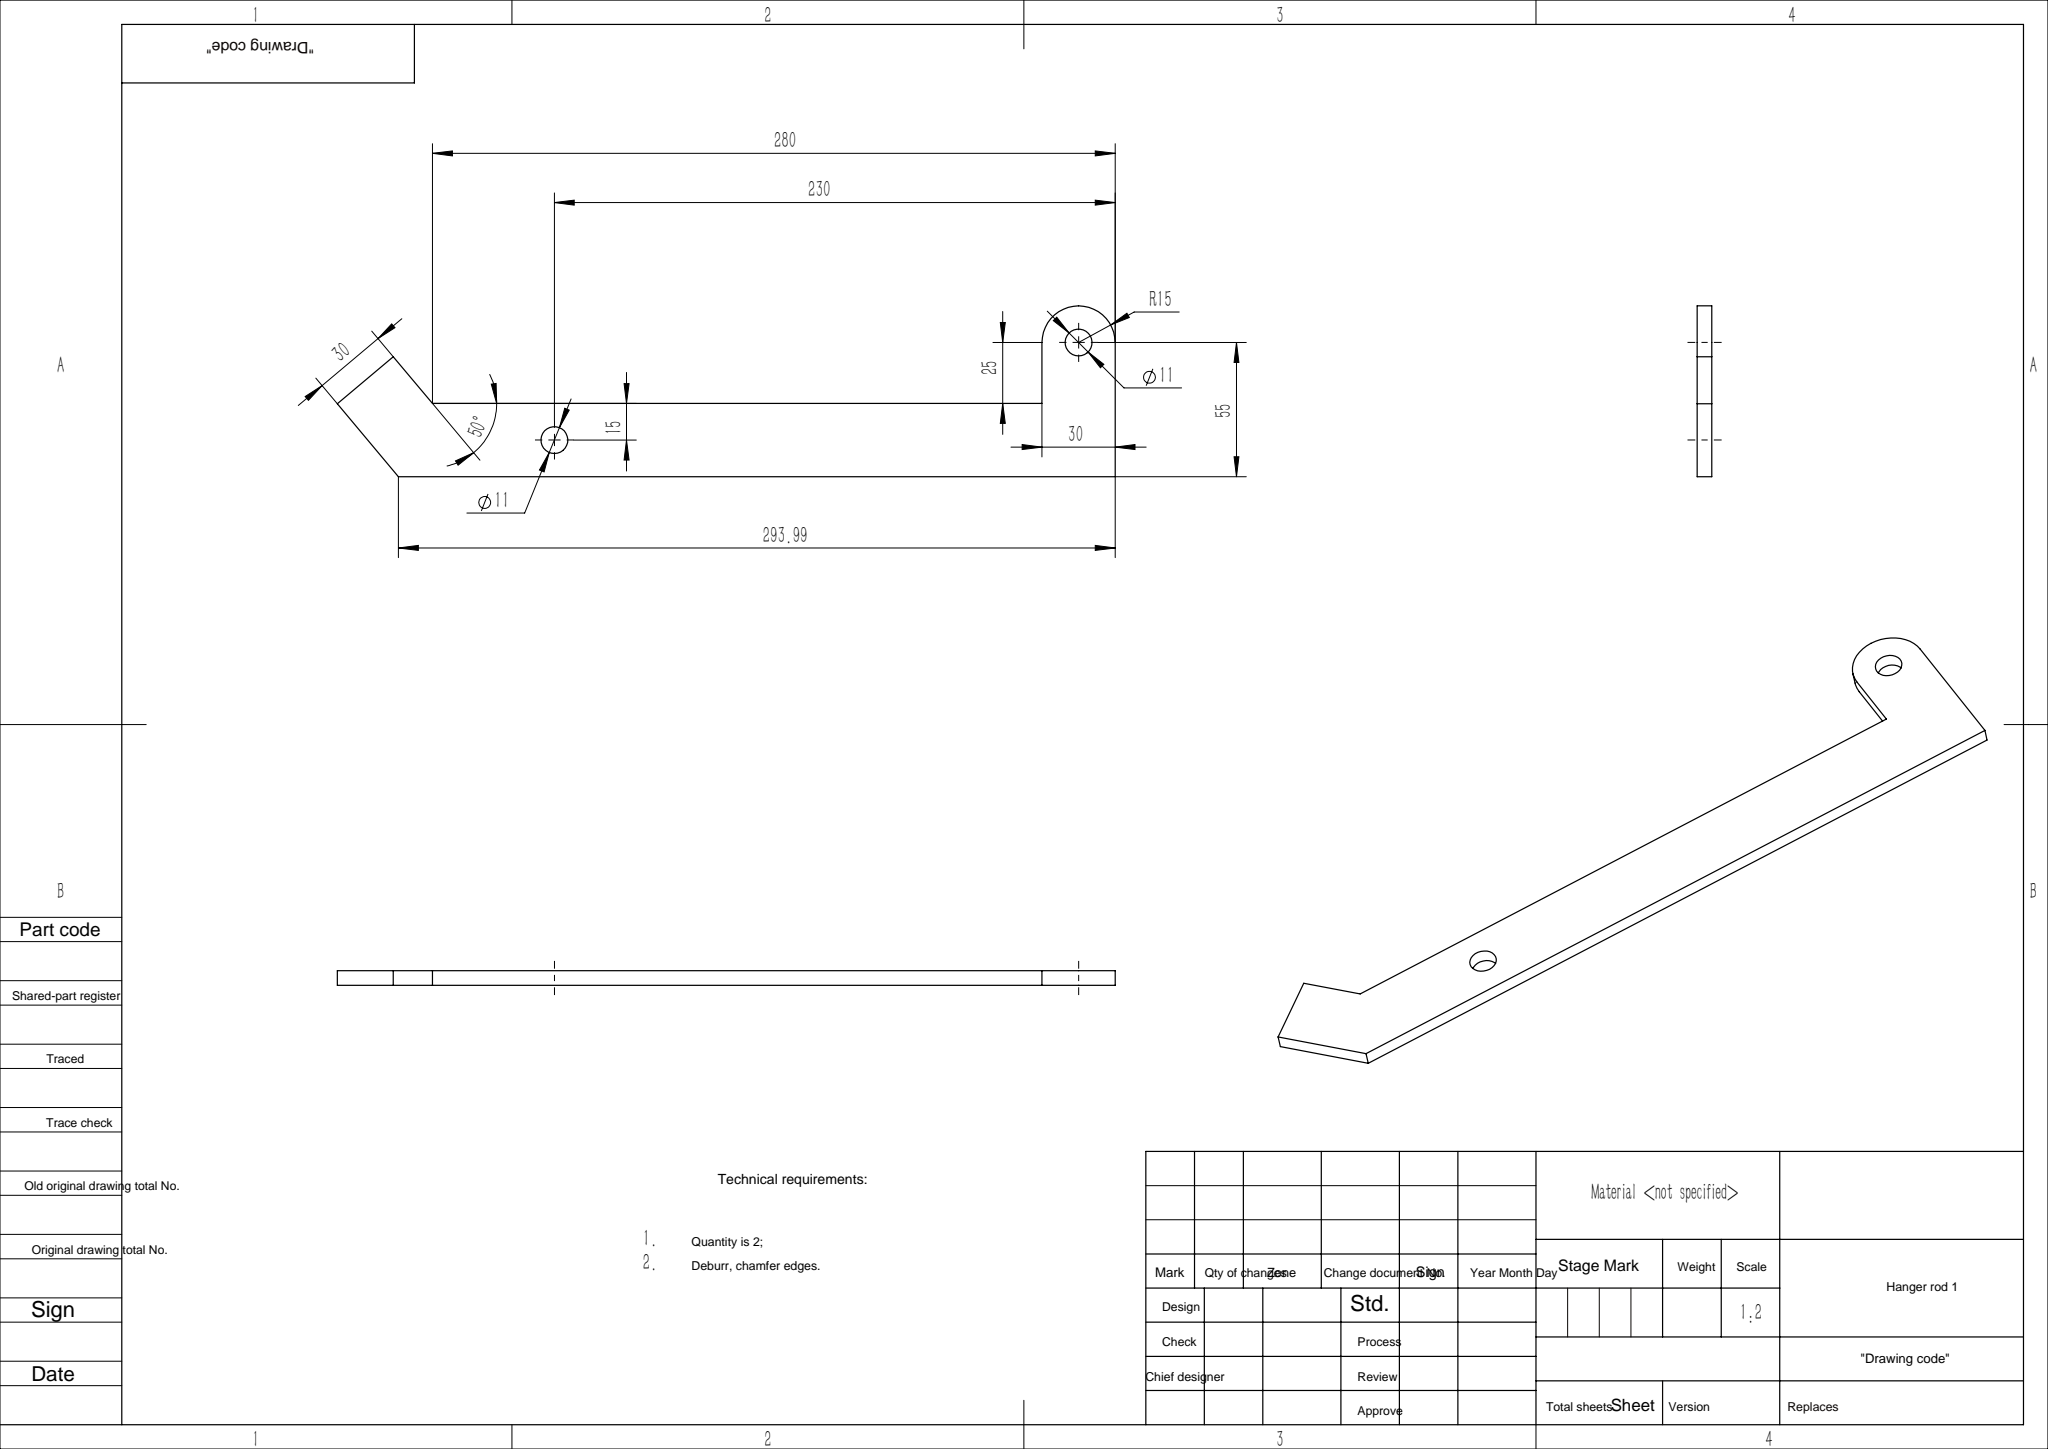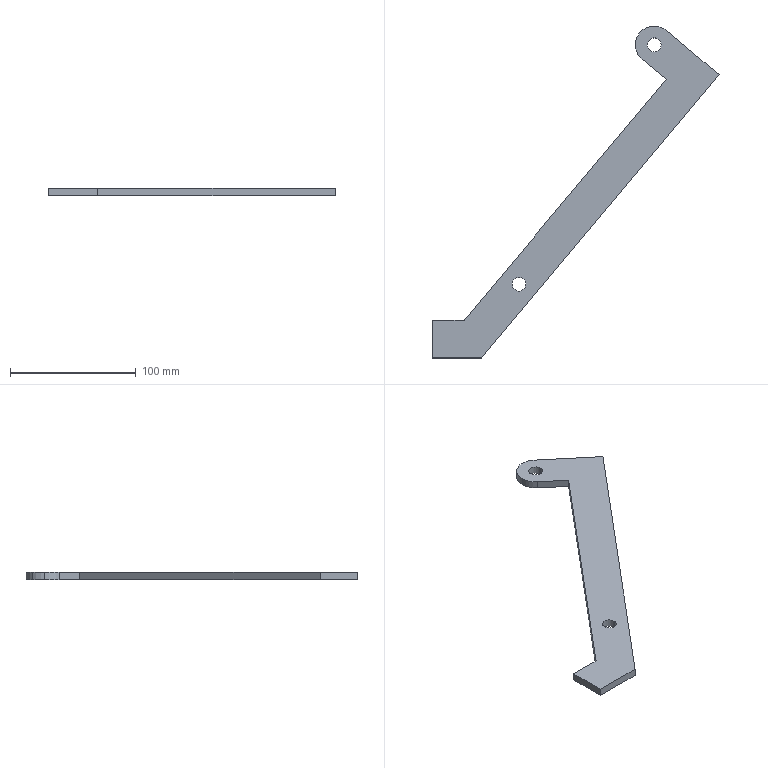Part | SolidWorks | features Extrusion 1, Fillet 1 | 1 solid | 16 faces | box 227.962 x 264.071 x 6 mm | volume 62898 mm3 | plane 9 | cylinder 7 | commonest cylinder face diameters 11 x4 30 x3
STEP:
#1=CARTESIAN_POINT('',(124.697,228.713,6.));
#2=VERTEX_POINT('',#1);
#3=CARTESIAN_POINT('',(130.055,217.223,6.));
#4=VERTEX_POINT('',#3);
#5=CARTESIAN_POINT('',(139.697,228.713,6.));
#6=DIRECTION('',(0.,0.,1.));
#7=DIRECTION('',(1.,0.,0.));
#8=AXIS2_PLACEMENT_3D('',#5,#6,#7);
#9=CIRCLE('',#8,15.);
#10=EDGE_CURVE('',#2,#4,#9,.T.);
#11=ORIENTED_EDGE('',*,*,#10,.F.);
#12=CARTESIAN_POINT('',(124.697,228.713,0.));
#13=VERTEX_POINT('',#12);
#14=CARTESIAN_POINT('',(124.697,228.713,6.));
#15=DIRECTION('',(0.,0.,-1.));
#16=VECTOR('',#15,1000.);
#17=LINE('',#14,#16);
#18=EDGE_CURVE('',#2,#13,#17,.T.);
#19=ORIENTED_EDGE('',*,*,#18,.T.);
#20=CARTESIAN_POINT('',(130.055,217.223,0.));
#21=VERTEX_POINT('',#20);
#22=CARTESIAN_POINT('',(139.697,228.713,0.));
#23=DIRECTION('',(0.,0.,-1.));
#24=DIRECTION('',(1.,0.,0.));
#25=AXIS2_PLACEMENT_3D('',#22,#23,#24);
#26=CIRCLE('',#25,15.);
#27=EDGE_CURVE('',#21,#13,#26,.T.);
#28=ORIENTED_EDGE('',*,*,#27,.F.);
#29=CARTESIAN_POINT('',(130.055,217.223,6.));
#30=DIRECTION('',(0.,0.,-1.));
#31=VECTOR('',#30,1000.);
#32=LINE('',#29,#31);
#33=EDGE_CURVE('',#4,#21,#32,.T.);
#34=ORIENTED_EDGE('',*,*,#33,.F.);
#35=EDGE_LOOP('',(#11,#19,#28,#34));
#36=FACE_OUTER_BOUND('',#35,.T.);
#37=CARTESIAN_POINT('',(139.697,228.713,6.));
#38=DIRECTION('',(0.,0.,-1.));
#39=DIRECTION('',(-1.,0.,0.));
#40=AXIS2_PLACEMENT_3D('',#37,#38,#39);
#41=CYLINDRICAL_SURFACE('',#40,15.);
#42=ADVANCED_FACE('',(#36),#41,.T.);
#43=CARTESIAN_POINT('',(26.639,38.302,6.));
#44=VERTEX_POINT('',#43);
#45=CARTESIAN_POINT('',(37.639,38.302,6.));
#46=VERTEX_POINT('',#45);
#47=CARTESIAN_POINT('',(32.139,38.302,6.));
#48=DIRECTION('',(0.,0.,1.));
#49=DIRECTION('',(1.,0.,0.));
#50=AXIS2_PLACEMENT_3D('',#47,#48,#49);
#51=CIRCLE('',#50,5.5);
#52=EDGE_CURVE('',#44,#46,#51,.T.);
#53=ORIENTED_EDGE('',*,*,#52,.T.);
#54=CARTESIAN_POINT('',(37.639,38.302,0.));
#55=VERTEX_POINT('',#54);
#56=CARTESIAN_POINT('',(37.639,38.302,6.));
#57=DIRECTION('',(0.,0.,-1.));
#58=VECTOR('',#57,1000.);
#59=LINE('',#56,#58);
#60=EDGE_CURVE('',#46,#55,#59,.T.);
#61=ORIENTED_EDGE('',*,*,#60,.T.);
#62=CARTESIAN_POINT('',(26.639,38.302,0.));
#63=VERTEX_POINT('',#62);
#64=CARTESIAN_POINT('',(32.139,38.302,0.));
#65=DIRECTION('',(0.,0.,1.));
#66=DIRECTION('',(1.,0.,0.));
#67=AXIS2_PLACEMENT_3D('',#64,#65,#66);
#68=CIRCLE('',#67,5.5);
#69=EDGE_CURVE('',#63,#55,#68,.T.);
#70=ORIENTED_EDGE('',*,*,#69,.F.);
#71=CARTESIAN_POINT('',(26.639,38.302,6.));
#72=DIRECTION('',(0.,0.,-1.));
#73=VECTOR('',#72,1000.);
#74=LINE('',#71,#73);
#75=EDGE_CURVE('',#44,#63,#74,.T.);
#76=ORIENTED_EDGE('',*,*,#75,.F.);
#77=EDGE_LOOP('',(#53,#61,#70,#76));
#78=FACE_OUTER_BOUND('',#77,.T.);
#79=CARTESIAN_POINT('',(32.139,38.302,6.));
#80=DIRECTION('',(0.,0.,-1.));
#81=DIRECTION('',(-1.,0.,0.));
#82=AXIS2_PLACEMENT_3D('',#79,#80,#81);
#83=CYLINDRICAL_SURFACE('',#82,5.5);
#84=ADVANCED_FACE('',(#78),#83,.F.);
#85=CARTESIAN_POINT('',(134.197,228.713,6.));
#86=VERTEX_POINT('',#85);
#87=CARTESIAN_POINT('',(145.197,228.713,6.));
#88=VERTEX_POINT('',#87);
#89=CARTESIAN_POINT('',(139.697,228.713,6.));
#90=DIRECTION('',(0.,0.,1.));
#91=DIRECTION('',(1.,0.,0.));
#92=AXIS2_PLACEMENT_3D('',#89,#90,#91);
#93=CIRCLE('',#92,5.5);
#94=EDGE_CURVE('',#86,#88,#93,.T.);
#95=ORIENTED_EDGE('',*,*,#94,.T.);
#96=CARTESIAN_POINT('',(145.197,228.713,0.));
#97=VERTEX_POINT('',#96);
#98=CARTESIAN_POINT('',(145.197,228.713,6.));
#99=DIRECTION('',(0.,0.,-1.));
#100=VECTOR('',#99,1000.);
#101=LINE('',#98,#100);
#102=EDGE_CURVE('',#88,#97,#101,.T.);
#103=ORIENTED_EDGE('',*,*,#102,.T.);
#104=CARTESIAN_POINT('',(134.197,228.713,0.));
#105=VERTEX_POINT('',#104);
#106=CARTESIAN_POINT('',(139.697,228.713,0.));
#107=DIRECTION('',(0.,0.,1.));
#108=DIRECTION('',(1.,0.,0.));
#109=AXIS2_PLACEMENT_3D('',#106,#107,#108);
#110=CIRCLE('',#109,5.5);
#111=EDGE_CURVE('',#105,#97,#110,.T.);
#112=ORIENTED_EDGE('',*,*,#111,.F.);
#113=CARTESIAN_POINT('',(134.197,228.713,6.));
#114=DIRECTION('',(0.,0.,-1.));
#115=VECTOR('',#114,1000.);
#116=LINE('',#113,#115);
#117=EDGE_CURVE('',#86,#105,#116,.T.);
#118=ORIENTED_EDGE('',*,*,#117,.F.);
#119=EDGE_LOOP('',(#95,#103,#112,#118));
#120=FACE_OUTER_BOUND('',#119,.T.);
#121=CARTESIAN_POINT('',(139.697,228.713,6.));
#122=DIRECTION('',(0.,0.,-1.));
#123=DIRECTION('',(-1.,0.,0.));
#124=AXIS2_PLACEMENT_3D('',#121,#122,#123);
#125=CYLINDRICAL_SURFACE('',#124,5.5);
#126=ADVANCED_FACE('',(#120),#125,.F.);
#127=ORIENTED_EDGE('',*,*,#94,.F.);
#128=CARTESIAN_POINT('',(139.697,228.713,6.));
#129=DIRECTION('',(0.,0.,1.));
#130=DIRECTION('',(1.,0.,0.));
#131=AXIS2_PLACEMENT_3D('',#128,#129,#130);
#132=CIRCLE('',#131,5.5);
#133=EDGE_CURVE('',#88,#86,#132,.T.);
#134=ORIENTED_EDGE('',*,*,#133,.F.);
#135=EDGE_LOOP('',(#127,#134));
#136=FACE_BOUND('',#135,.T.);
#137=CARTESIAN_POINT('',(149.339,240.204,6.));
#138=VERTEX_POINT('',#137);
#139=CARTESIAN_POINT('',(128.206,238.355,6.));
#140=VERTEX_POINT('',#139);
#141=CARTESIAN_POINT('',(139.697,228.713,6.));
#142=DIRECTION('',(0.,0.,1.));
#143=DIRECTION('',(1.,0.,0.));
#144=AXIS2_PLACEMENT_3D('',#141,#142,#143);
#145=CIRCLE('',#144,15.);
#146=EDGE_CURVE('',#138,#140,#145,.T.);
#147=ORIENTED_EDGE('',*,*,#146,.T.);
#148=CARTESIAN_POINT('',(139.697,228.713,6.));
#149=DIRECTION('',(0.,0.,1.));
#150=DIRECTION('',(1.,0.,0.));
#151=AXIS2_PLACEMENT_3D('',#148,#149,#150);
#152=CIRCLE('',#151,15.);
#153=EDGE_CURVE('',#140,#2,#152,.T.);
#154=ORIENTED_EDGE('',*,*,#153,.T.);
#155=ORIENTED_EDGE('',*,*,#10,.T.);
#156=CARTESIAN_POINT('',(149.206,201.153,6.));
#157=VERTEX_POINT('',#156);
#158=CARTESIAN_POINT('',(141.546,207.581,6.));
#159=DIRECTION('',(0.766,-0.6428,0.));
#160=VECTOR('',#159,1000.);
#161=LINE('',#158,#160);
#162=EDGE_CURVE('',#4,#157,#161,.T.);
#163=ORIENTED_EDGE('',*,*,#162,.T.);
#164=CARTESIAN_POINT('',(-11.491,9.642,6.));
#165=VERTEX_POINT('',#164);
#166=CARTESIAN_POINT('',(-11.491,9.642,6.));
#167=DIRECTION('',(-0.6428,-0.766,0.));
#168=VECTOR('',#167,1000.);
#169=LINE('',#166,#168);
#170=EDGE_CURVE('',#157,#165,#169,.T.);
#171=ORIENTED_EDGE('',*,*,#170,.T.);
#172=CARTESIAN_POINT('',(-36.491,9.642,6.));
#173=VERTEX_POINT('',#172);
#174=CARTESIAN_POINT('',(-11.491,9.642,6.));
#175=DIRECTION('',(-1.,0.,0.));
#176=VECTOR('',#175,1000.);
#177=LINE('',#174,#176);
#178=EDGE_CURVE('',#165,#173,#177,.T.);
#179=ORIENTED_EDGE('',*,*,#178,.T.);
#180=CARTESIAN_POINT('',(-36.491,-20.358,6.));
#181=VERTEX_POINT('',#180);
#182=CARTESIAN_POINT('',(-36.491,9.642,6.));
#183=DIRECTION('',(0.,-1.,0.));
#184=VECTOR('',#183,1000.);
#185=LINE('',#182,#184);
#186=EDGE_CURVE('',#173,#181,#185,.T.);
#187=ORIENTED_EDGE('',*,*,#186,.T.);
#188=CARTESIAN_POINT('',(2.499,-20.358,6.));
#189=VERTEX_POINT('',#188);
#190=CARTESIAN_POINT('',(-36.491,-20.358,6.));
#191=DIRECTION('',(1.,0.,0.));
#192=VECTOR('',#191,1000.);
#193=LINE('',#190,#192);
#194=EDGE_CURVE('',#181,#189,#193,.T.);
#195=ORIENTED_EDGE('',*,*,#194,.T.);
#196=CARTESIAN_POINT('',(191.471,204.851,6.));
#197=VERTEX_POINT('',#196);
#198=CARTESIAN_POINT('',(172.188,181.869,6.));
#199=DIRECTION('',(0.6428,0.766,0.));
#200=VECTOR('',#199,1000.);
#201=LINE('',#198,#200);
#202=EDGE_CURVE('',#189,#197,#201,.T.);
#203=ORIENTED_EDGE('',*,*,#202,.T.);
#204=CARTESIAN_POINT('',(191.471,204.851,6.));
#205=DIRECTION('',(-0.766,0.6428,0.));
#206=VECTOR('',#205,1000.);
#207=LINE('',#204,#206);
#208=EDGE_CURVE('',#197,#138,#207,.T.);
#209=ORIENTED_EDGE('',*,*,#208,.T.);
#210=EDGE_LOOP('',(#147,#154,#155,#163,#171,#179,#187,#195,#203,#209));
#211=FACE_OUTER_BOUND('',#210,.T.);
#212=ORIENTED_EDGE('',*,*,#52,.F.);
#213=CARTESIAN_POINT('',(32.139,38.302,6.));
#214=DIRECTION('',(0.,0.,1.));
#215=DIRECTION('',(1.,0.,0.));
#216=AXIS2_PLACEMENT_3D('',#213,#214,#215);
#217=CIRCLE('',#216,5.5);
#218=EDGE_CURVE('',#46,#44,#217,.T.);
#219=ORIENTED_EDGE('',*,*,#218,.F.);
#220=EDGE_LOOP('',(#212,#219));
#221=FACE_BOUND('',#220,.T.);
#222=CARTESIAN_POINT('',(0.,0.,6.));
#223=DIRECTION('',(0.,0.,1.));
#224=DIRECTION('',(1.,0.,0.));
#225=AXIS2_PLACEMENT_3D('',#222,#223,#224);
#226=PLANE('',#225);
#227=ADVANCED_FACE('',(#136,#211,#221),#226,.T.);
#228=ORIENTED_EDGE('',*,*,#111,.T.);
#229=CARTESIAN_POINT('',(139.697,228.713,0.));
#230=DIRECTION('',(0.,0.,1.));
#231=DIRECTION('',(1.,0.,0.));
#232=AXIS2_PLACEMENT_3D('',#229,#230,#231);
#233=CIRCLE('',#232,5.5);
#234=EDGE_CURVE('',#97,#105,#233,.T.);
#235=ORIENTED_EDGE('',*,*,#234,.T.);
#236=EDGE_LOOP('',(#228,#235));
#237=FACE_BOUND('',#236,.T.);
#238=CARTESIAN_POINT('',(149.206,201.153,0.));
#239=VERTEX_POINT('',#238);
#240=CARTESIAN_POINT('',(149.206,201.153,0.));
#241=DIRECTION('',(0.766,-0.6428,0.));
#242=VECTOR('',#241,1000.);
#243=LINE('',#240,#242);
#244=EDGE_CURVE('',#21,#239,#243,.T.);
#245=ORIENTED_EDGE('',*,*,#244,.F.);
#246=ORIENTED_EDGE('',*,*,#27,.T.);
#247=CARTESIAN_POINT('',(128.206,238.355,0.));
#248=VERTEX_POINT('',#247);
#249=CARTESIAN_POINT('',(139.697,228.713,0.));
#250=DIRECTION('',(0.,0.,-1.));
#251=DIRECTION('',(1.,0.,0.));
#252=AXIS2_PLACEMENT_3D('',#249,#250,#251);
#253=CIRCLE('',#252,15.);
#254=EDGE_CURVE('',#13,#248,#253,.T.);
#255=ORIENTED_EDGE('',*,*,#254,.T.);
#256=CARTESIAN_POINT('',(149.339,240.204,0.));
#257=VERTEX_POINT('',#256);
#258=CARTESIAN_POINT('',(139.697,228.713,0.));
#259=DIRECTION('',(0.,0.,-1.));
#260=DIRECTION('',(1.,0.,0.));
#261=AXIS2_PLACEMENT_3D('',#258,#259,#260);
#262=CIRCLE('',#261,15.);
#263=EDGE_CURVE('',#248,#257,#262,.T.);
#264=ORIENTED_EDGE('',*,*,#263,.T.);
#265=CARTESIAN_POINT('',(191.471,204.851,0.));
#266=VERTEX_POINT('',#265);
#267=CARTESIAN_POINT('',(191.471,204.851,0.));
#268=DIRECTION('',(-0.766,0.6428,0.));
#269=VECTOR('',#268,1000.);
#270=LINE('',#267,#269);
#271=EDGE_CURVE('',#266,#257,#270,.T.);
#272=ORIENTED_EDGE('',*,*,#271,.F.);
#273=CARTESIAN_POINT('',(2.499,-20.358,0.));
#274=VERTEX_POINT('',#273);
#275=CARTESIAN_POINT('',(2.499,-20.358,0.));
#276=DIRECTION('',(0.6428,0.766,0.));
#277=VECTOR('',#276,1000.);
#278=LINE('',#275,#277);
#279=EDGE_CURVE('',#274,#266,#278,.T.);
#280=ORIENTED_EDGE('',*,*,#279,.F.);
#281=CARTESIAN_POINT('',(-36.491,-20.358,0.));
#282=VERTEX_POINT('',#281);
#283=CARTESIAN_POINT('',(-36.491,-20.358,0.));
#284=DIRECTION('',(1.,0.,0.));
#285=VECTOR('',#284,1000.);
#286=LINE('',#283,#285);
#287=EDGE_CURVE('',#282,#274,#286,.T.);
#288=ORIENTED_EDGE('',*,*,#287,.F.);
#289=CARTESIAN_POINT('',(-36.491,9.642,0.));
#290=VERTEX_POINT('',#289);
#291=CARTESIAN_POINT('',(-36.491,9.642,0.));
#292=DIRECTION('',(0.,-1.,0.));
#293=VECTOR('',#292,1000.);
#294=LINE('',#291,#293);
#295=EDGE_CURVE('',#290,#282,#294,.T.);
#296=ORIENTED_EDGE('',*,*,#295,.F.);
#297=CARTESIAN_POINT('',(-11.491,9.642,0.));
#298=VERTEX_POINT('',#297);
#299=CARTESIAN_POINT('',(-11.491,9.642,0.));
#300=DIRECTION('',(-1.,0.,0.));
#301=VECTOR('',#300,1000.);
#302=LINE('',#299,#301);
#303=EDGE_CURVE('',#298,#290,#302,.T.);
#304=ORIENTED_EDGE('',*,*,#303,.F.);
#305=CARTESIAN_POINT('',(-11.491,9.642,0.));
#306=DIRECTION('',(-0.6428,-0.766,0.));
#307=VECTOR('',#306,1000.);
#308=LINE('',#305,#307);
#309=EDGE_CURVE('',#239,#298,#308,.T.);
#310=ORIENTED_EDGE('',*,*,#309,.F.);
#311=EDGE_LOOP('',(#245,#246,#255,#264,#272,#280,#288,#296,#304,#310));
#312=FACE_OUTER_BOUND('',#311,.T.);
#313=ORIENTED_EDGE('',*,*,#69,.T.);
#314=CARTESIAN_POINT('',(32.139,38.302,0.));
#315=DIRECTION('',(0.,0.,1.));
#316=DIRECTION('',(1.,0.,0.));
#317=AXIS2_PLACEMENT_3D('',#314,#315,#316);
#318=CIRCLE('',#317,5.5);
#319=EDGE_CURVE('',#55,#63,#318,.T.);
#320=ORIENTED_EDGE('',*,*,#319,.T.);
#321=EDGE_LOOP('',(#313,#320));
#322=FACE_BOUND('',#321,.T.);
#323=CARTESIAN_POINT('',(0.,0.,0.));
#324=DIRECTION('',(0.,0.,1.));
#325=DIRECTION('',(1.,0.,0.));
#326=AXIS2_PLACEMENT_3D('',#323,#324,#325);
#327=PLANE('',#326);
#328=ADVANCED_FACE('',(#237,#312,#322),#327,.F.);
#329=ORIENTED_EDGE('',*,*,#271,.T.);
#330=CARTESIAN_POINT('',(149.339,240.204,6.));
#331=DIRECTION('',(0.,0.,1.));
#332=VECTOR('',#331,1000.);
#333=LINE('',#330,#332);
#334=EDGE_CURVE('',#257,#138,#333,.T.);
#335=ORIENTED_EDGE('',*,*,#334,.T.);
#336=ORIENTED_EDGE('',*,*,#208,.F.);
#337=CARTESIAN_POINT('',(191.471,204.851,6.));
#338=DIRECTION('',(0.,0.,-1.));
#339=VECTOR('',#338,1000.);
#340=LINE('',#337,#339);
#341=EDGE_CURVE('',#197,#266,#340,.T.);
#342=ORIENTED_EDGE('',*,*,#341,.T.);
#343=EDGE_LOOP('',(#329,#335,#336,#342));
#344=FACE_OUTER_BOUND('',#343,.T.);
#345=CARTESIAN_POINT('',(191.471,204.851,6.));
#346=DIRECTION('',(-0.6428,-0.766,0.));
#347=DIRECTION('',(0.766,-0.6428,0.));
#348=AXIS2_PLACEMENT_3D('',#345,#346,#347);
#349=PLANE('',#348);
#350=ADVANCED_FACE('',(#344),#349,.F.);
#351=ORIENTED_EDGE('',*,*,#162,.F.);
#352=ORIENTED_EDGE('',*,*,#33,.T.);
#353=ORIENTED_EDGE('',*,*,#244,.T.);
#354=CARTESIAN_POINT('',(149.206,201.153,6.));
#355=DIRECTION('',(0.,0.,-1.));
#356=VECTOR('',#355,1000.);
#357=LINE('',#354,#356);
#358=EDGE_CURVE('',#157,#239,#357,.T.);
#359=ORIENTED_EDGE('',*,*,#358,.F.);
#360=EDGE_LOOP('',(#351,#352,#353,#359));
#361=FACE_OUTER_BOUND('',#360,.T.);
#362=CARTESIAN_POINT('',(149.206,201.153,6.));
#363=DIRECTION('',(0.6428,0.766,0.));
#364=DIRECTION('',(-0.766,0.6428,0.));
#365=AXIS2_PLACEMENT_3D('',#362,#363,#364);
#366=PLANE('',#365);
#367=ADVANCED_FACE('',(#361),#366,.F.);
#368=ORIENTED_EDGE('',*,*,#309,.T.);
#369=CARTESIAN_POINT('',(-11.491,9.642,6.));
#370=DIRECTION('',(0.,0.,-1.));
#371=VECTOR('',#370,1000.);
#372=LINE('',#369,#371);
#373=EDGE_CURVE('',#165,#298,#372,.T.);
#374=ORIENTED_EDGE('',*,*,#373,.F.);
#375=ORIENTED_EDGE('',*,*,#170,.F.);
#376=ORIENTED_EDGE('',*,*,#358,.T.);
#377=EDGE_LOOP('',(#368,#374,#375,#376));
#378=FACE_OUTER_BOUND('',#377,.T.);
#379=CARTESIAN_POINT('',(-11.491,9.642,6.));
#380=DIRECTION('',(0.766,-0.6428,0.));
#381=DIRECTION('',(0.6428,0.766,0.));
#382=AXIS2_PLACEMENT_3D('',#379,#380,#381);
#383=PLANE('',#382);
#384=ADVANCED_FACE('',(#378),#383,.F.);
#385=ORIENTED_EDGE('',*,*,#303,.T.);
#386=CARTESIAN_POINT('',(-36.491,9.642,6.));
#387=DIRECTION('',(0.,0.,-1.));
#388=VECTOR('',#387,1000.);
#389=LINE('',#386,#388);
#390=EDGE_CURVE('',#173,#290,#389,.T.);
#391=ORIENTED_EDGE('',*,*,#390,.F.);
#392=ORIENTED_EDGE('',*,*,#178,.F.);
#393=ORIENTED_EDGE('',*,*,#373,.T.);
#394=EDGE_LOOP('',(#385,#391,#392,#393));
#395=FACE_OUTER_BOUND('',#394,.T.);
#396=CARTESIAN_POINT('',(-11.491,9.642,6.));
#397=DIRECTION('',(0.,-1.,0.));
#398=DIRECTION('',(1.,0.,0.));
#399=AXIS2_PLACEMENT_3D('',#396,#397,#398);
#400=PLANE('',#399);
#401=ADVANCED_FACE('',(#395),#400,.F.);
#402=ORIENTED_EDGE('',*,*,#295,.T.);
#403=CARTESIAN_POINT('',(-36.491,-20.358,6.));
#404=DIRECTION('',(0.,0.,-1.));
#405=VECTOR('',#404,1000.);
#406=LINE('',#403,#405);
#407=EDGE_CURVE('',#181,#282,#406,.T.);
#408=ORIENTED_EDGE('',*,*,#407,.F.);
#409=ORIENTED_EDGE('',*,*,#186,.F.);
#410=ORIENTED_EDGE('',*,*,#390,.T.);
#411=EDGE_LOOP('',(#402,#408,#409,#410));
#412=FACE_OUTER_BOUND('',#411,.T.);
#413=CARTESIAN_POINT('',(-36.491,9.642,6.));
#414=DIRECTION('',(1.,0.,0.));
#415=DIRECTION('',(0.,0.,-1.));
#416=AXIS2_PLACEMENT_3D('',#413,#414,#415);
#417=PLANE('',#416);
#418=ADVANCED_FACE('',(#412),#417,.F.);
#419=ORIENTED_EDGE('',*,*,#287,.T.);
#420=CARTESIAN_POINT('',(2.499,-20.358,6.));
#421=DIRECTION('',(0.,0.,-1.));
#422=VECTOR('',#421,1000.);
#423=LINE('',#420,#422);
#424=EDGE_CURVE('',#189,#274,#423,.T.);
#425=ORIENTED_EDGE('',*,*,#424,.F.);
#426=ORIENTED_EDGE('',*,*,#194,.F.);
#427=ORIENTED_EDGE('',*,*,#407,.T.);
#428=EDGE_LOOP('',(#419,#425,#426,#427));
#429=FACE_OUTER_BOUND('',#428,.T.);
#430=CARTESIAN_POINT('',(-36.491,-20.358,6.));
#431=DIRECTION('',(0.,1.,0.));
#432=DIRECTION('',(-1.,0.,0.));
#433=AXIS2_PLACEMENT_3D('',#430,#431,#432);
#434=PLANE('',#433);
#435=ADVANCED_FACE('',(#429),#434,.F.);
#436=ORIENTED_EDGE('',*,*,#279,.T.);
#437=ORIENTED_EDGE('',*,*,#341,.F.);
#438=ORIENTED_EDGE('',*,*,#202,.F.);
#439=ORIENTED_EDGE('',*,*,#424,.T.);
#440=EDGE_LOOP('',(#436,#437,#438,#439));
#441=FACE_OUTER_BOUND('',#440,.T.);
#442=CARTESIAN_POINT('',(2.499,-20.358,6.));
#443=DIRECTION('',(-0.766,0.6428,0.));
#444=DIRECTION('',(-0.6428,-0.766,0.));
#445=AXIS2_PLACEMENT_3D('',#442,#443,#444);
#446=PLANE('',#445);
#447=ADVANCED_FACE('',(#441),#446,.F.);
#448=ORIENTED_EDGE('',*,*,#102,.F.);
#449=ORIENTED_EDGE('',*,*,#133,.T.);
#450=ORIENTED_EDGE('',*,*,#117,.T.);
#451=ORIENTED_EDGE('',*,*,#234,.F.);
#452=EDGE_LOOP('',(#448,#449,#450,#451));
#453=FACE_OUTER_BOUND('',#452,.T.);
#454=CARTESIAN_POINT('',(139.697,228.713,6.));
#455=DIRECTION('',(0.,0.,-1.));
#456=DIRECTION('',(-1.,0.,0.));
#457=AXIS2_PLACEMENT_3D('',#454,#455,#456);
#458=CYLINDRICAL_SURFACE('',#457,5.5);
#459=ADVANCED_FACE('',(#453),#458,.F.);
#460=ORIENTED_EDGE('',*,*,#60,.F.);
#461=ORIENTED_EDGE('',*,*,#218,.T.);
#462=ORIENTED_EDGE('',*,*,#75,.T.);
#463=ORIENTED_EDGE('',*,*,#319,.F.);
#464=EDGE_LOOP('',(#460,#461,#462,#463));
#465=FACE_OUTER_BOUND('',#464,.T.);
#466=CARTESIAN_POINT('',(32.139,38.302,6.));
#467=DIRECTION('',(0.,0.,-1.));
#468=DIRECTION('',(-1.,0.,0.));
#469=AXIS2_PLACEMENT_3D('',#466,#467,#468);
#470=CYLINDRICAL_SURFACE('',#469,5.5);
#471=ADVANCED_FACE('',(#465),#470,.F.);
#472=CARTESIAN_POINT('',(128.206,238.355,6.));
#473=DIRECTION('',(0.,0.,-1.));
#474=VECTOR('',#473,1000.);
#475=LINE('',#472,#474);
#476=EDGE_CURVE('',#140,#248,#475,.T.);
#477=ORIENTED_EDGE('',*,*,#476,.F.);
#478=ORIENTED_EDGE('',*,*,#146,.F.);
#479=ORIENTED_EDGE('',*,*,#334,.F.);
#480=ORIENTED_EDGE('',*,*,#263,.F.);
#481=EDGE_LOOP('',(#477,#478,#479,#480));
#482=FACE_OUTER_BOUND('',#481,.T.);
#483=CARTESIAN_POINT('',(139.697,228.713,6.));
#484=DIRECTION('',(0.,0.,-1.));
#485=DIRECTION('',(-1.,0.,0.));
#486=AXIS2_PLACEMENT_3D('',#483,#484,#485);
#487=CYLINDRICAL_SURFACE('',#486,15.);
#488=ADVANCED_FACE('',(#482),#487,.T.);
#489=ORIENTED_EDGE('',*,*,#18,.F.);
#490=ORIENTED_EDGE('',*,*,#153,.F.);
#491=ORIENTED_EDGE('',*,*,#476,.T.);
#492=ORIENTED_EDGE('',*,*,#254,.F.);
#493=EDGE_LOOP('',(#489,#490,#491,#492));
#494=FACE_OUTER_BOUND('',#493,.T.);
#495=CARTESIAN_POINT('',(139.697,228.713,6.));
#496=DIRECTION('',(0.,0.,-1.));
#497=DIRECTION('',(-1.,0.,0.));
#498=AXIS2_PLACEMENT_3D('',#495,#496,#497);
#499=CYLINDRICAL_SURFACE('',#498,15.);
#500=ADVANCED_FACE('',(#494),#499,.T.);
#501=CLOSED_SHELL('',(#42,#84,#126,#227,#328,#350,#367,#384,#401,#418,#435,#447,#459,#471,#488,#500));
#502=MANIFOLD_SOLID_BREP('',#501);
#503=CARTESIAN_POINT('',(0.,0.,0.));
#504=DIRECTION('',(0.,0.,1.));
#505=DIRECTION('',(1.,0.,0.));
#506=AXIS2_PLACEMENT_3D('',#503,#504,#505);
#507=(LENGTH_UNIT()NAMED_UNIT(*)SI_UNIT(.MILLI.,.METRE.));
#508=UNCERTAINTY_MEASURE_WITH_UNIT(LENGTH_MEASURE(0.00001),#507,'','');
#509=(NAMED_UNIT(*)PLANE_ANGLE_UNIT()SI_UNIT($,.RADIAN.));
#510=(NAMED_UNIT(*)SI_UNIT($,.STERADIAN.)SOLID_ANGLE_UNIT());
#511=(GEOMETRIC_REPRESENTATION_CONTEXT(3)GLOBAL_UNCERTAINTY_ASSIGNED_CONTEXT((#508))GLOBAL_UNIT_ASSIGNED_CONTEXT((#507,#509,#510))REPRESENTATION_CONTEXT('',''));
#512=ADVANCED_BREP_SHAPE_REPRESENTATION('',(#502,#506),#511);